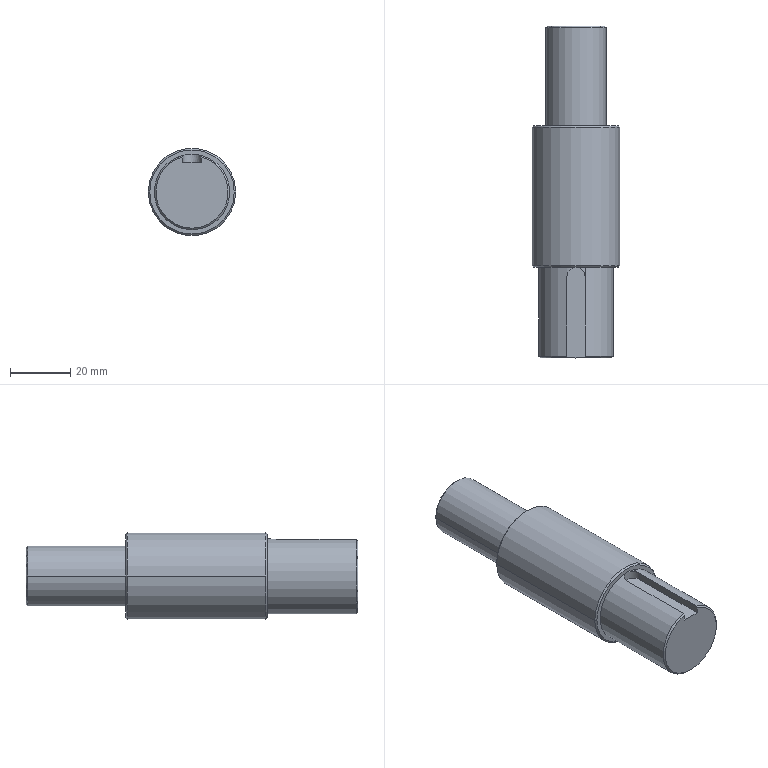Part | Creo | features DATUM PLANE 3, CURVE 2, CHAMFER 1, COORDINATE SYSTEM 1, CUT 1, PROTRUSION 1, ROUND 1 | 1 solid | 21 faces | box 29 x 110.003 x 29 mm | volume 55617 mm3 | plane 7 | cylinder 7 | cone 7 | commonest cylinder face diameters 20 x2 25 x2 29 x2 6 x1
STEP:
#1=CARTESIAN_POINT('',(0.,0.,0.));
#2=DIRECTION('',(0.,0.,1.));
#3=DIRECTION('',(1.,0.,0.));
#4=AXIS2_PLACEMENT_3D('',#1,#2,#3);
#5=CARTESIAN_POINT('',(14.,30.,0.));
#6=VERTEX_POINT('',#5);
#7=CARTESIAN_POINT('',(-14.,30.,0.));
#8=VERTEX_POINT('',#7);
#9=CARTESIAN_POINT('',(0.,30.,0.));
#10=DIRECTION('',(0.,1.,0.));
#11=DIRECTION('',(1.,0.,0.));
#12=AXIS2_PLACEMENT_3D('',#9,#10,#11);
#13=CIRCLE('',#12,14.);
#14=EDGE_CURVE('',#6,#8,#13,.T.);
#15=ORIENTED_EDGE('',*,*,#14,.T.);
#16=CARTESIAN_POINT('',(0.,30.,0.));
#17=DIRECTION('',(0.,1.,0.));
#18=DIRECTION('',(-1.,0.,0.));
#19=AXIS2_PLACEMENT_3D('',#16,#17,#18);
#20=CIRCLE('',#19,14.);
#21=EDGE_CURVE('',#8,#6,#20,.T.);
#22=ORIENTED_EDGE('',*,*,#21,.T.);
#23=EDGE_LOOP('',(#15,#22));
#24=FACE_OUTER_BOUND('',#23,.F.);
#25=CARTESIAN_POINT('',(3.,30.,12.135));
#26=VERTEX_POINT('',#25);
#27=CARTESIAN_POINT('',(0.,30.,12.5));
#28=VERTEX_POINT('',#27);
#29=CARTESIAN_POINT('',(0.,30.,0.));
#30=DIRECTION('',(0.,1.,0.));
#31=DIRECTION('',(0.24,0.,0.9708));
#32=AXIS2_PLACEMENT_3D('',#29,#30,#31);
#33=CIRCLE('',#32,12.5);
#34=EDGE_CURVE('',#26,#28,#33,.T.);
#35=ORIENTED_EDGE('',*,*,#34,.F.);
#36=CARTESIAN_POINT('',(0.,30.,0.));
#37=DIRECTION('',(0.,1.,0.));
#38=DIRECTION('',(0.,0.,1.));
#39=AXIS2_PLACEMENT_3D('',#36,#37,#38);
#40=CIRCLE('',#39,12.5);
#41=EDGE_CURVE('',#28,#26,#40,.T.);
#42=ORIENTED_EDGE('',*,*,#41,.F.);
#43=EDGE_LOOP('',(#35,#42));
#44=FACE_BOUND('',#43,.F.);
#45=CARTESIAN_POINT('',(0.,30.,0.));
#46=DIRECTION('',(0.,1.,0.));
#47=DIRECTION('',(1.,0.,0.));
#48=AXIS2_PLACEMENT_3D('',#45,#46,#47);
#49=PLANE('',#48);
#50=ADVANCED_FACE('',(#24,#44),#49,.F.);
#51=CARTESIAN_POINT('',(3.,0.5,12.135));
#52=VERTEX_POINT('',#51);
#53=CARTESIAN_POINT('',(-3.,0.5,12.135));
#54=VERTEX_POINT('',#53);
#55=CARTESIAN_POINT('',(0.000000139,0.5,0.0001994));
#56=DIRECTION('',(0.,1.,0.));
#57=DIRECTION('',(0.24,0.,0.9708));
#58=AXIS2_PLACEMENT_3D('',#55,#56,#57);
#59=CIRCLE('',#58,12.5);
#60=EDGE_CURVE('',#52,#54,#59,.T.);
#61=ORIENTED_EDGE('',*,*,#60,.F.);
#62=CARTESIAN_POINT('',(3.,27.,12.135));
#63=VERTEX_POINT('',#62);
#64=CARTESIAN_POINT('',(3.,0.5,12.135));
#65=DIRECTION('',(-0.000000297,1.,-0.000001201));
#66=VECTOR('',#65,26.5);
#67=LINE('',#64,#66);
#68=EDGE_CURVE('',#52,#63,#67,.T.);
#69=ORIENTED_EDGE('',*,*,#68,.T.);
#70=CARTESIAN_POINT('',(3.,27.,12.135));
#71=DIRECTION('',(0.,1.,0.));
#72=VECTOR('',#71,3.);
#73=LINE('',#70,#72);
#74=EDGE_CURVE('',#63,#26,#73,.T.);
#75=ORIENTED_EDGE('',*,*,#74,.T.);
#76=ORIENTED_EDGE('',*,*,#34,.T.);
#77=CARTESIAN_POINT('',(-3.,27.,12.135));
#78=VERTEX_POINT('',#77);
#79=CARTESIAN_POINT('',(-3.,27.,12.135));
#80=CARTESIAN_POINT('',(-3.,27.259,12.135));
#81=CARTESIAN_POINT('',(-2.933,27.778,12.152));
#82=CARTESIAN_POINT('',(-2.63,28.514,12.222));
#83=CARTESIAN_POINT('',(-2.146,29.146,12.319));
#84=CARTESIAN_POINT('',(-1.514,29.63,12.414));
#85=CARTESIAN_POINT('',(-0.7784,29.933,12.484));
#86=CARTESIAN_POINT('',(-0.2587,30.,12.5));
#87=CARTESIAN_POINT('',(0.,30.,12.5));
#88=B_SPLINE_CURVE_WITH_KNOTS('',3,(#79,#80,#81,#82,#83,#84,#85,#86,#87),.UNSPECIFIED.,.F.,.F.,(4,1,1,1,1,1,4),(0.,0.1667,0.3333,0.5,0.6667,0.8333,1.),.UNSPECIFIED.);
#89=EDGE_CURVE('',#78,#28,#88,.T.);
#90=ORIENTED_EDGE('',*,*,#89,.F.);
#91=CARTESIAN_POINT('',(-3.,0.5,12.135));
#92=DIRECTION('',(-0.000000332,1.,-0.000001199));
#93=VECTOR('',#92,26.5);
#94=LINE('',#91,#93);
#95=EDGE_CURVE('',#54,#78,#94,.T.);
#96=ORIENTED_EDGE('',*,*,#95,.F.);
#97=EDGE_LOOP('',(#61,#69,#75,#76,#90,#96));
#98=FACE_OUTER_BOUND('',#97,.F.);
#99=CARTESIAN_POINT('',(0.,0.,0.));
#100=DIRECTION('',(0.,1.,0.));
#101=DIRECTION('',(1.,0.,0.));
#102=AXIS2_PLACEMENT_3D('',#99,#100,#101);
#103=CYLINDRICAL_SURFACE('',#102,12.5);
#104=ADVANCED_FACE('',(#98),#103,.T.);
#105=ORIENTED_EDGE('',*,*,#60,.T.);
#106=CARTESIAN_POINT('',(-3.,-0.00003545,11.619));
#107=VERTEX_POINT('',#106);
#108=CARTESIAN_POINT('',(-3.,0.4153,12.047));
#109=CARTESIAN_POINT('',(-3.,0.2472,11.874));
#110=CARTESIAN_POINT('',(-3.,0.08196,11.704));
#111=B_SPLINE_CURVE_WITH_KNOTS('',3,(#53,#108,#109,#110,#106),.UNSPECIFIED.,.F.,.F.,(4,1,4),(0.,0.5,1.),.UNSPECIFIED.);
#112=EDGE_CURVE('',#54,#107,#111,.T.);
#113=ORIENTED_EDGE('',*,*,#112,.T.);
#114=CARTESIAN_POINT('',(3.,-0.00003132,11.619));
#115=VERTEX_POINT('',#114);
#116=CARTESIAN_POINT('',(0.000000139,0.,0.0001994));
#117=DIRECTION('',(0.,-1.,0.));
#118=DIRECTION('',(-0.25,0.,0.9682));
#119=AXIS2_PLACEMENT_3D('',#116,#117,#118);
#120=CIRCLE('',#119,12.);
#121=EDGE_CURVE('',#107,#115,#120,.T.);
#122=ORIENTED_EDGE('',*,*,#121,.T.);
#123=CARTESIAN_POINT('',(3.,0.08194,11.704));
#124=CARTESIAN_POINT('',(3.,0.2471,11.874));
#125=CARTESIAN_POINT('',(3.,0.4153,12.047));
#126=B_SPLINE_CURVE_WITH_KNOTS('',3,(#114,#123,#124,#125,#51),.UNSPECIFIED.,.F.,.F.,(4,1,4),(0.,0.5,1.),.UNSPECIFIED.);
#127=EDGE_CURVE('',#115,#52,#126,.T.);
#128=ORIENTED_EDGE('',*,*,#127,.T.);
#129=EDGE_LOOP('',(#105,#113,#122,#128));
#130=FACE_OUTER_BOUND('',#129,.F.);
#131=CARTESIAN_POINT('',(0.000000139,0.25,0.0001994));
#132=DIRECTION('',(0.,1.,0.));
#133=DIRECTION('',(0.,0.,-1.));
#134=AXIS2_PLACEMENT_3D('',#131,#132,#133);
#135=CONICAL_SURFACE('',#134,12.25,45.);
#136=ADVANCED_FACE('',(#130),#135,.T.);
#137=ORIENTED_EDGE('',*,*,#112,.F.);
#138=ORIENTED_EDGE('',*,*,#95,.T.);
#139=CARTESIAN_POINT('',(-3.,27.,9.635));
#140=VERTEX_POINT('',#139);
#141=CARTESIAN_POINT('',(-3.,27.,9.635));
#142=DIRECTION('',(0.,0.,1.));
#143=VECTOR('',#142,2.5);
#144=LINE('',#141,#143);
#145=EDGE_CURVE('',#140,#78,#144,.T.);
#146=ORIENTED_EDGE('',*,*,#145,.F.);
#147=CARTESIAN_POINT('',(-3.,0.,9.635));
#148=VERTEX_POINT('',#147);
#149=CARTESIAN_POINT('',(-3.,0.,9.635));
#150=DIRECTION('',(0.,1.,0.));
#151=VECTOR('',#150,27.);
#152=LINE('',#149,#151);
#153=EDGE_CURVE('',#148,#140,#152,.T.);
#154=ORIENTED_EDGE('',*,*,#153,.F.);
#155=CARTESIAN_POINT('',(-3.,-0.00003545,11.619));
#156=DIRECTION('',(-0.000004434,0.00001787,-1.));
#157=VECTOR('',#156,1.984);
#158=LINE('',#155,#157);
#159=EDGE_CURVE('',#107,#148,#158,.T.);
#160=ORIENTED_EDGE('',*,*,#159,.F.);
#161=EDGE_LOOP('',(#137,#138,#146,#154,#160));
#162=FACE_OUTER_BOUND('',#161,.F.);
#163=CARTESIAN_POINT('',(-3.,0.,12.135));
#164=DIRECTION('',(-1.,0.,0.));
#165=DIRECTION('',(0.,0.,-1.));
#166=AXIS2_PLACEMENT_3D('',#163,#164,#165);
#167=PLANE('',#166);
#168=ADVANCED_FACE('',(#162),#167,.F.);
#169=CARTESIAN_POINT('',(3.,27.,9.635));
#170=VERTEX_POINT('',#169);
#171=CARTESIAN_POINT('',(3.,27.,12.135));
#172=DIRECTION('',(0.,0.,-1.));
#173=VECTOR('',#172,2.5);
#174=LINE('',#171,#173);
#175=EDGE_CURVE('',#63,#170,#174,.T.);
#176=ORIENTED_EDGE('',*,*,#175,.T.);
#177=CARTESIAN_POINT('',(0.,27.,9.635));
#178=DIRECTION('',(0.,0.,-1.));
#179=DIRECTION('',(-1.,0.,0.));
#180=AXIS2_PLACEMENT_3D('',#177,#178,#179);
#181=CIRCLE('',#180,3.);
#182=EDGE_CURVE('',#140,#170,#181,.T.);
#183=ORIENTED_EDGE('',*,*,#182,.F.);
#184=ORIENTED_EDGE('',*,*,#145,.T.);
#185=ORIENTED_EDGE('',*,*,#89,.T.);
#186=CARTESIAN_POINT('',(0.,30.,12.5));
#187=CARTESIAN_POINT('',(0.2587,30.,12.5));
#188=CARTESIAN_POINT('',(0.7784,29.933,12.484));
#189=CARTESIAN_POINT('',(1.514,29.63,12.414));
#190=CARTESIAN_POINT('',(2.146,29.146,12.319));
#191=CARTESIAN_POINT('',(2.63,28.514,12.222));
#192=CARTESIAN_POINT('',(2.933,27.778,12.152));
#193=CARTESIAN_POINT('',(3.,27.259,12.135));
#194=CARTESIAN_POINT('',(3.,27.,12.135));
#195=B_SPLINE_CURVE_WITH_KNOTS('',3,(#186,#187,#188,#189,#190,#191,#192,#193,#194),.UNSPECIFIED.,.F.,.F.,(4,1,1,1,1,1,4),(0.,0.1667,0.3333,0.5,0.6667,0.8333,1.),.UNSPECIFIED.);
#196=EDGE_CURVE('',#28,#63,#195,.T.);
#197=ORIENTED_EDGE('',*,*,#196,.T.);
#198=EDGE_LOOP('',(#176,#183,#184,#185,#197));
#199=FACE_OUTER_BOUND('',#198,.F.);
#200=CARTESIAN_POINT('',(0.,27.,52.369));
#201=DIRECTION('',(0.,0.,-1.));
#202=DIRECTION('',(0.,1.,0.));
#203=AXIS2_PLACEMENT_3D('',#200,#201,#202);
#204=CYLINDRICAL_SURFACE('',#203,3.);
#205=ADVANCED_FACE('',(#199),#204,.F.);
#206=ORIENTED_EDGE('',*,*,#127,.F.);
#207=CARTESIAN_POINT('',(3.,0.,9.635));
#208=VERTEX_POINT('',#207);
#209=CARTESIAN_POINT('',(3.,0.,9.635));
#210=DIRECTION('',(0.000003946,-0.00001578,1.));
#211=VECTOR('',#210,1.984);
#212=LINE('',#209,#211);
#213=EDGE_CURVE('',#208,#115,#212,.T.);
#214=ORIENTED_EDGE('',*,*,#213,.F.);
#215=CARTESIAN_POINT('',(3.,0.,9.635));
#216=DIRECTION('',(0.,1.,0.));
#217=VECTOR('',#216,27.);
#218=LINE('',#215,#217);
#219=EDGE_CURVE('',#208,#170,#218,.T.);
#220=ORIENTED_EDGE('',*,*,#219,.T.);
#221=ORIENTED_EDGE('',*,*,#175,.F.);
#222=ORIENTED_EDGE('',*,*,#68,.F.);
#223=EDGE_LOOP('',(#206,#214,#220,#221,#222));
#224=FACE_OUTER_BOUND('',#223,.F.);
#225=CARTESIAN_POINT('',(3.,0.,9.635));
#226=DIRECTION('',(1.,0.,0.));
#227=DIRECTION('',(0.,0.,1.));
#228=AXIS2_PLACEMENT_3D('',#225,#226,#227);
#229=PLANE('',#228);
#230=ADVANCED_FACE('',(#224),#229,.F.);
#231=ORIENTED_EDGE('',*,*,#121,.F.);
#232=ORIENTED_EDGE('',*,*,#159,.T.);
#233=CARTESIAN_POINT('',(-3.,0.,9.635));
#234=DIRECTION('',(1.,0.,0.));
#235=VECTOR('',#234,6.);
#236=LINE('',#233,#235);
#237=EDGE_CURVE('',#148,#208,#236,.T.);
#238=ORIENTED_EDGE('',*,*,#237,.T.);
#239=ORIENTED_EDGE('',*,*,#213,.T.);
#240=EDGE_LOOP('',(#231,#232,#238,#239));
#241=FACE_OUTER_BOUND('',#240,.F.);
#242=CARTESIAN_POINT('',(0.,0.,0.));
#243=DIRECTION('',(0.,1.,0.));
#244=DIRECTION('',(1.,0.,0.));
#245=AXIS2_PLACEMENT_3D('',#242,#243,#244);
#246=PLANE('',#245);
#247=ADVANCED_FACE('',(#241),#246,.F.);
#248=ORIENTED_EDGE('',*,*,#182,.T.);
#249=ORIENTED_EDGE('',*,*,#219,.F.);
#250=ORIENTED_EDGE('',*,*,#237,.F.);
#251=ORIENTED_EDGE('',*,*,#153,.T.);
#252=EDGE_LOOP('',(#248,#249,#250,#251));
#253=FACE_OUTER_BOUND('',#252,.F.);
#254=CARTESIAN_POINT('',(-3.,0.,9.635));
#255=DIRECTION('',(0.,0.,-1.));
#256=DIRECTION('',(1.,0.,0.));
#257=AXIS2_PLACEMENT_3D('',#254,#255,#256);
#258=PLANE('',#257);
#259=ADVANCED_FACE('',(#253),#258,.F.);
#260=ORIENTED_EDGE('',*,*,#41,.T.);
#261=ORIENTED_EDGE('',*,*,#74,.F.);
#262=ORIENTED_EDGE('',*,*,#196,.F.);
#263=EDGE_LOOP('',(#260,#261,#262));
#264=FACE_OUTER_BOUND('',#263,.F.);
#265=CARTESIAN_POINT('',(0.,0.,0.));
#266=DIRECTION('',(0.,1.,0.));
#267=DIRECTION('',(1.,0.,0.));
#268=AXIS2_PLACEMENT_3D('',#265,#266,#267);
#269=CYLINDRICAL_SURFACE('',#268,12.5);
#270=ADVANCED_FACE('',(#264),#269,.T.);
#271=CARTESIAN_POINT('',(14.5,30.5,0.));
#272=VERTEX_POINT('',#271);
#273=CARTESIAN_POINT('',(-14.5,30.5,0.));
#274=VERTEX_POINT('',#273);
#275=CARTESIAN_POINT('',(0.,30.5,0.));
#276=DIRECTION('',(0.,1.,0.));
#277=DIRECTION('',(1.,0.,0.));
#278=AXIS2_PLACEMENT_3D('',#275,#276,#277);
#279=CIRCLE('',#278,14.5);
#280=EDGE_CURVE('',#272,#274,#279,.T.);
#281=ORIENTED_EDGE('',*,*,#280,.T.);
#282=CARTESIAN_POINT('',(-14.5,30.5,-0.000000002));
#283=DIRECTION('',(0.7071,-0.7071,-0.000000001));
#284=VECTOR('',#283,0.7071);
#285=LINE('',#282,#284);
#286=EDGE_CURVE('',#274,#8,#285,.T.);
#287=ORIENTED_EDGE('',*,*,#286,.T.);
#288=ORIENTED_EDGE('',*,*,#14,.F.);
#289=CARTESIAN_POINT('',(14.5,30.5,0.000000002));
#290=DIRECTION('',(-0.7071,-0.7071,0.000000001));
#291=VECTOR('',#290,0.7071);
#292=LINE('',#289,#291);
#293=EDGE_CURVE('',#272,#6,#292,.T.);
#294=ORIENTED_EDGE('',*,*,#293,.F.);
#295=EDGE_LOOP('',(#281,#287,#288,#294));
#296=FACE_OUTER_BOUND('',#295,.F.);
#297=CARTESIAN_POINT('',(0.,30.25,0.));
#298=DIRECTION('',(0.,1.,0.));
#299=DIRECTION('',(0.,0.,-1.));
#300=AXIS2_PLACEMENT_3D('',#297,#298,#299);
#301=CONICAL_SURFACE('',#300,14.25,45.);
#302=ADVANCED_FACE('',(#296),#301,.T.);
#303=ORIENTED_EDGE('',*,*,#280,.F.);
#304=CARTESIAN_POINT('',(14.5,76.503,0.));
#305=VERTEX_POINT('',#304);
#306=CARTESIAN_POINT('',(14.5,30.5,0.000000002));
#307=DIRECTION('',(0.,1.,0.));
#308=VECTOR('',#307,46.003);
#309=LINE('',#306,#308);
#310=EDGE_CURVE('',#272,#305,#309,.T.);
#311=ORIENTED_EDGE('',*,*,#310,.T.);
#312=CARTESIAN_POINT('',(-14.5,76.503,0.));
#313=VERTEX_POINT('',#312);
#314=CARTESIAN_POINT('',(0.,76.503,0.));
#315=DIRECTION('',(0.,1.,0.));
#316=DIRECTION('',(1.,0.,0.));
#317=AXIS2_PLACEMENT_3D('',#314,#315,#316);
#318=CIRCLE('',#317,14.5);
#319=EDGE_CURVE('',#305,#313,#318,.T.);
#320=ORIENTED_EDGE('',*,*,#319,.T.);
#321=CARTESIAN_POINT('',(-14.5,30.5,-0.000000002));
#322=DIRECTION('',(0.,1.,0.));
#323=VECTOR('',#322,46.003);
#324=LINE('',#321,#323);
#325=EDGE_CURVE('',#274,#313,#324,.T.);
#326=ORIENTED_EDGE('',*,*,#325,.F.);
#327=EDGE_LOOP('',(#303,#311,#320,#326));
#328=FACE_OUTER_BOUND('',#327,.F.);
#329=CARTESIAN_POINT('',(0.,0.,0.));
#330=DIRECTION('',(0.,1.,0.));
#331=DIRECTION('',(1.,0.,0.));
#332=AXIS2_PLACEMENT_3D('',#329,#330,#331);
#333=CYLINDRICAL_SURFACE('',#332,14.5);
#334=ADVANCED_FACE('',(#328),#333,.T.);
#335=CARTESIAN_POINT('',(0.,30.5,0.));
#336=DIRECTION('',(0.,1.,0.));
#337=DIRECTION('',(-1.,0.,0.));
#338=AXIS2_PLACEMENT_3D('',#335,#336,#337);
#339=CIRCLE('',#338,14.5);
#340=EDGE_CURVE('',#274,#272,#339,.T.);
#341=ORIENTED_EDGE('',*,*,#340,.F.);
#342=ORIENTED_EDGE('',*,*,#325,.T.);
#343=CARTESIAN_POINT('',(0.,76.503,0.));
#344=DIRECTION('',(0.,1.,0.));
#345=DIRECTION('',(-1.,0.,0.));
#346=AXIS2_PLACEMENT_3D('',#343,#344,#345);
#347=CIRCLE('',#346,14.5);
#348=EDGE_CURVE('',#313,#305,#347,.T.);
#349=ORIENTED_EDGE('',*,*,#348,.T.);
#350=ORIENTED_EDGE('',*,*,#310,.F.);
#351=EDGE_LOOP('',(#341,#342,#349,#350));
#352=FACE_OUTER_BOUND('',#351,.F.);
#353=CARTESIAN_POINT('',(0.,0.,0.));
#354=DIRECTION('',(0.,1.,0.));
#355=DIRECTION('',(1.,0.,0.));
#356=AXIS2_PLACEMENT_3D('',#353,#354,#355);
#357=CYLINDRICAL_SURFACE('',#356,14.5);
#358=ADVANCED_FACE('',(#352),#357,.T.);
#359=ORIENTED_EDGE('',*,*,#340,.T.);
#360=ORIENTED_EDGE('',*,*,#293,.T.);
#361=ORIENTED_EDGE('',*,*,#21,.F.);
#362=ORIENTED_EDGE('',*,*,#286,.F.);
#363=EDGE_LOOP('',(#359,#360,#361,#362));
#364=FACE_OUTER_BOUND('',#363,.F.);
#365=CARTESIAN_POINT('',(0.,30.25,0.));
#366=DIRECTION('',(0.,1.,0.));
#367=DIRECTION('',(0.,0.,-1.));
#368=AXIS2_PLACEMENT_3D('',#365,#366,#367);
#369=CONICAL_SURFACE('',#368,14.25,45.);
#370=ADVANCED_FACE('',(#364),#369,.T.);
#371=CARTESIAN_POINT('',(-14.,77.003,0.));
#372=VERTEX_POINT('',#371);
#373=CARTESIAN_POINT('',(14.,77.003,0.));
#374=VERTEX_POINT('',#373);
#375=CARTESIAN_POINT('',(0.,77.003,0.));
#376=DIRECTION('',(0.,1.,0.));
#377=DIRECTION('',(-1.,0.,0.));
#378=AXIS2_PLACEMENT_3D('',#375,#376,#377);
#379=CIRCLE('',#378,14.);
#380=EDGE_CURVE('',#372,#374,#379,.T.);
#381=ORIENTED_EDGE('',*,*,#380,.T.);
#382=CARTESIAN_POINT('',(14.,77.003,-0.000000008));
#383=DIRECTION('',(0.7071,-0.7071,0.000000003));
#384=VECTOR('',#383,0.7071);
#385=LINE('',#382,#384);
#386=EDGE_CURVE('',#374,#305,#385,.T.);
#387=ORIENTED_EDGE('',*,*,#386,.T.);
#388=ORIENTED_EDGE('',*,*,#348,.F.);
#389=CARTESIAN_POINT('',(-14.,77.003,0.000000008));
#390=DIRECTION('',(-0.7071,-0.7071,-0.000000003));
#391=VECTOR('',#390,0.7071);
#392=LINE('',#389,#391);
#393=EDGE_CURVE('',#372,#313,#392,.T.);
#394=ORIENTED_EDGE('',*,*,#393,.F.);
#395=EDGE_LOOP('',(#381,#387,#388,#394));
#396=FACE_OUTER_BOUND('',#395,.F.);
#397=CARTESIAN_POINT('',(0.,76.753,0.));
#398=DIRECTION('',(0.,-1.,0.));
#399=DIRECTION('',(0.,0.,-1.));
#400=AXIS2_PLACEMENT_3D('',#397,#398,#399);
#401=CONICAL_SURFACE('',#400,14.25,45.);
#402=ADVANCED_FACE('',(#396),#401,.T.);
#403=CARTESIAN_POINT('',(0.,77.003,0.));
#404=DIRECTION('',(0.,1.,0.));
#405=DIRECTION('',(1.,0.,0.));
#406=AXIS2_PLACEMENT_3D('',#403,#404,#405);
#407=CIRCLE('',#406,14.);
#408=EDGE_CURVE('',#374,#372,#407,.T.);
#409=ORIENTED_EDGE('',*,*,#408,.F.);
#410=ORIENTED_EDGE('',*,*,#380,.F.);
#411=EDGE_LOOP('',(#409,#410));
#412=FACE_OUTER_BOUND('',#411,.F.);
#413=CARTESIAN_POINT('',(10.,77.003,0.));
#414=VERTEX_POINT('',#413);
#415=CARTESIAN_POINT('',(-10.,77.003,0.));
#416=VERTEX_POINT('',#415);
#417=CARTESIAN_POINT('',(0.,77.003,0.));
#418=DIRECTION('',(0.,1.,0.));
#419=DIRECTION('',(1.,0.,0.));
#420=AXIS2_PLACEMENT_3D('',#417,#418,#419);
#421=CIRCLE('',#420,10.);
#422=EDGE_CURVE('',#414,#416,#421,.T.);
#423=ORIENTED_EDGE('',*,*,#422,.T.);
#424=CARTESIAN_POINT('',(0.,77.003,0.));
#425=DIRECTION('',(0.,-1.,0.));
#426=DIRECTION('',(1.,0.,0.));
#427=AXIS2_PLACEMENT_3D('',#424,#425,#426);
#428=CIRCLE('',#427,10.);
#429=EDGE_CURVE('',#414,#416,#428,.T.);
#430=ORIENTED_EDGE('',*,*,#429,.F.);
#431=EDGE_LOOP('',(#423,#430));
#432=FACE_BOUND('',#431,.F.);
#433=CARTESIAN_POINT('',(0.,77.003,0.));
#434=DIRECTION('',(0.,1.,0.));
#435=DIRECTION('',(1.,0.,0.));
#436=AXIS2_PLACEMENT_3D('',#433,#434,#435);
#437=PLANE('',#436);
#438=ADVANCED_FACE('',(#412,#432),#437,.T.);
#439=CARTESIAN_POINT('',(10.,109.503,0.));
#440=VERTEX_POINT('',#439);
#441=CARTESIAN_POINT('',(-10.,109.503,0.));
#442=VERTEX_POINT('',#441);
#443=CARTESIAN_POINT('',(0.,109.503,0.));
#444=DIRECTION('',(0.,1.,0.));
#445=DIRECTION('',(1.,0.,0.));
#446=AXIS2_PLACEMENT_3D('',#443,#444,#445);
#447=CIRCLE('',#446,10.);
#448=EDGE_CURVE('',#440,#442,#447,.T.);
#449=ORIENTED_EDGE('',*,*,#448,.T.);
#450=CARTESIAN_POINT('',(-10.,77.003,0.));
#451=DIRECTION('',(0.,1.,0.));
#452=VECTOR('',#451,32.5);
#453=LINE('',#450,#452);
#454=EDGE_CURVE('',#416,#442,#453,.T.);
#455=ORIENTED_EDGE('',*,*,#454,.F.);
#456=ORIENTED_EDGE('',*,*,#422,.F.);
#457=CARTESIAN_POINT('',(10.,77.003,0.));
#458=DIRECTION('',(0.,1.,0.));
#459=VECTOR('',#458,32.5);
#460=LINE('',#457,#459);
#461=EDGE_CURVE('',#414,#440,#460,.T.);
#462=ORIENTED_EDGE('',*,*,#461,.T.);
#463=EDGE_LOOP('',(#449,#455,#456,#462));
#464=FACE_OUTER_BOUND('',#463,.F.);
#465=CARTESIAN_POINT('',(0.,0.,0.));
#466=DIRECTION('',(0.,1.,0.));
#467=DIRECTION('',(1.,0.,0.));
#468=AXIS2_PLACEMENT_3D('',#465,#466,#467);
#469=CYLINDRICAL_SURFACE('',#468,10.);
#470=ADVANCED_FACE('',(#464),#469,.T.);
#471=CARTESIAN_POINT('',(9.5,110.003,0.));
#472=VERTEX_POINT('',#471);
#473=CARTESIAN_POINT('',(-9.5,110.003,0.));
#474=VERTEX_POINT('',#473);
#475=CARTESIAN_POINT('',(0.,110.003,0.));
#476=DIRECTION('',(0.,1.,0.));
#477=DIRECTION('',(1.,0.,0.));
#478=AXIS2_PLACEMENT_3D('',#475,#476,#477);
#479=CIRCLE('',#478,9.5);
#480=EDGE_CURVE('',#472,#474,#479,.T.);
#481=ORIENTED_EDGE('',*,*,#480,.T.);
#482=CARTESIAN_POINT('',(-9.5,110.003,0.000000001));
#483=DIRECTION('',(-0.7071,-0.7071,0.));
#484=VECTOR('',#483,0.7071);
#485=LINE('',#482,#484);
#486=EDGE_CURVE('',#474,#442,#485,.T.);
#487=ORIENTED_EDGE('',*,*,#486,.T.);
#488=ORIENTED_EDGE('',*,*,#448,.F.);
#489=CARTESIAN_POINT('',(9.5,110.003,-0.000000001));
#490=DIRECTION('',(0.7071,-0.7071,0.));
#491=VECTOR('',#490,0.7071);
#492=LINE('',#489,#491);
#493=EDGE_CURVE('',#472,#440,#492,.T.);
#494=ORIENTED_EDGE('',*,*,#493,.F.);
#495=EDGE_LOOP('',(#481,#487,#488,#494));
#496=FACE_OUTER_BOUND('',#495,.F.);
#497=CARTESIAN_POINT('',(0.,109.753,0.));
#498=DIRECTION('',(0.,-1.,0.));
#499=DIRECTION('',(0.,0.,-1.));
#500=AXIS2_PLACEMENT_3D('',#497,#498,#499);
#501=CONICAL_SURFACE('',#500,9.75,45.);
#502=ADVANCED_FACE('',(#496),#501,.T.);
#503=ORIENTED_EDGE('',*,*,#480,.F.);
#504=CARTESIAN_POINT('',(0.,110.003,0.));
#505=DIRECTION('',(0.,1.,0.));
#506=DIRECTION('',(-1.,0.,0.));
#507=AXIS2_PLACEMENT_3D('',#504,#505,#506);
#508=CIRCLE('',#507,9.5);
#509=EDGE_CURVE('',#474,#472,#508,.T.);
#510=ORIENTED_EDGE('',*,*,#509,.F.);
#511=EDGE_LOOP('',(#503,#510));
#512=FACE_OUTER_BOUND('',#511,.F.);
#513=CARTESIAN_POINT('',(0.,110.003,0.));
#514=DIRECTION('',(0.,1.,0.));
#515=DIRECTION('',(1.,0.,0.));
#516=AXIS2_PLACEMENT_3D('',#513,#514,#515);
#517=PLANE('',#516);
#518=ADVANCED_FACE('',(#512),#517,.T.);
#519=ORIENTED_EDGE('',*,*,#509,.T.);
#520=ORIENTED_EDGE('',*,*,#493,.T.);
#521=CARTESIAN_POINT('',(0.,109.503,0.));
#522=DIRECTION('',(0.,1.,0.));
#523=DIRECTION('',(-1.,0.,0.));
#524=AXIS2_PLACEMENT_3D('',#521,#522,#523);
#525=CIRCLE('',#524,10.);
#526=EDGE_CURVE('',#442,#440,#525,.T.);
#527=ORIENTED_EDGE('',*,*,#526,.F.);
#528=ORIENTED_EDGE('',*,*,#486,.F.);
#529=EDGE_LOOP('',(#519,#520,#527,#528));
#530=FACE_OUTER_BOUND('',#529,.F.);
#531=CARTESIAN_POINT('',(0.,109.753,0.));
#532=DIRECTION('',(0.,-1.,0.));
#533=DIRECTION('',(0.,0.,-1.));
#534=AXIS2_PLACEMENT_3D('',#531,#532,#533);
#535=CONICAL_SURFACE('',#534,9.75,45.);
#536=ADVANCED_FACE('',(#530),#535,.T.);
#537=ORIENTED_EDGE('',*,*,#526,.T.);
#538=ORIENTED_EDGE('',*,*,#461,.F.);
#539=ORIENTED_EDGE('',*,*,#429,.T.);
#540=ORIENTED_EDGE('',*,*,#454,.T.);
#541=EDGE_LOOP('',(#537,#538,#539,#540));
#542=FACE_OUTER_BOUND('',#541,.F.);
#543=CARTESIAN_POINT('',(0.,0.,0.));
#544=DIRECTION('',(0.,1.,0.));
#545=DIRECTION('',(1.,0.,0.));
#546=AXIS2_PLACEMENT_3D('',#543,#544,#545);
#547=CYLINDRICAL_SURFACE('',#546,10.);
#548=ADVANCED_FACE('',(#542),#547,.T.);
#549=ORIENTED_EDGE('',*,*,#408,.T.);
#550=ORIENTED_EDGE('',*,*,#393,.T.);
#551=ORIENTED_EDGE('',*,*,#319,.F.);
#552=ORIENTED_EDGE('',*,*,#386,.F.);
#553=EDGE_LOOP('',(#549,#550,#551,#552));
#554=FACE_OUTER_BOUND('',#553,.F.);
#555=CARTESIAN_POINT('',(0.,76.753,0.));
#556=DIRECTION('',(0.,-1.,0.));
#557=DIRECTION('',(0.,0.,-1.));
#558=AXIS2_PLACEMENT_3D('',#555,#556,#557);
#559=CONICAL_SURFACE('',#558,14.25,45.);
#560=ADVANCED_FACE('',(#554),#559,.T.);
#561=CLOSED_SHELL('',(#50,#104,#136,#168,#205,#230,#247,#259,#270,#302,#334,#358,#370,#402,#438,#470,#502,#518,#536,#548,#560));
#562=MANIFOLD_SOLID_BREP('',#561);
#563=(LENGTH_UNIT()NAMED_UNIT(*)SI_UNIT(.MILLI.,.METRE.));
#564=UNCERTAINTY_MEASURE_WITH_UNIT(LENGTH_MEASURE(0.01174),#563,'','');
#565=(NAMED_UNIT(*)PLANE_ANGLE_UNIT()SI_UNIT($,.RADIAN.));
#566=PLANE_ANGLE_MEASURE_WITH_UNIT(PLANE_ANGLE_MEASURE(0.01745),#565);
#567=(CONVERSION_BASED_UNIT('DEGREE',#566)NAMED_UNIT(*)PLANE_ANGLE_UNIT());
#568=(NAMED_UNIT(*)SI_UNIT($,.STERADIAN.)SOLID_ANGLE_UNIT());
#569=(GEOMETRIC_REPRESENTATION_CONTEXT(3)GLOBAL_UNCERTAINTY_ASSIGNED_CONTEXT((#564))GLOBAL_UNIT_ASSIGNED_CONTEXT((#563,#567,#568))REPRESENTATION_CONTEXT('',''));
#570=ADVANCED_BREP_SHAPE_REPRESENTATION('',(#4,#562),#569);